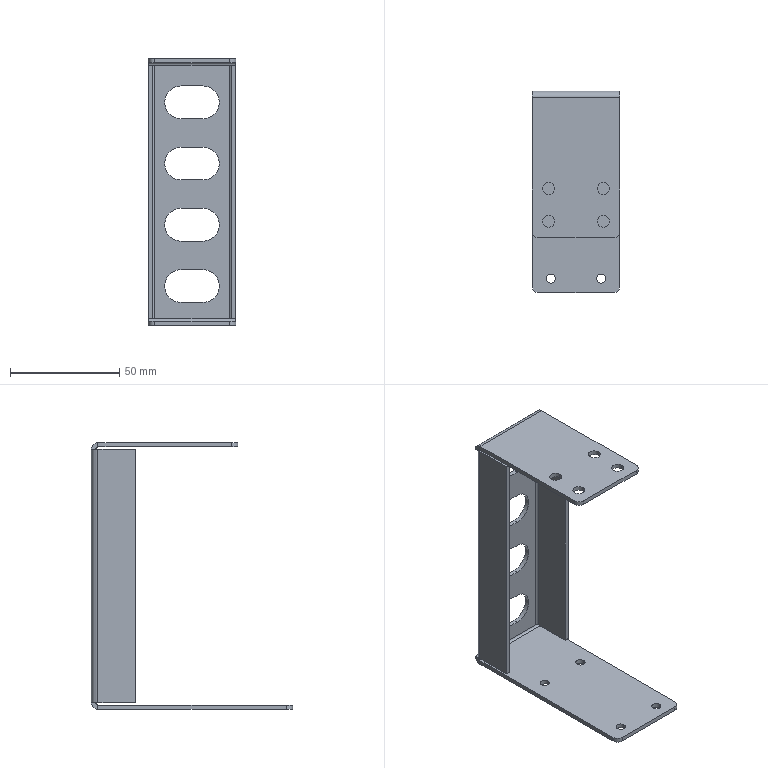Part | SolidWorks | features HoleWzd 2, EdgeFlange 1, Fillet 1, FlatPattern 1, ICE 1, LPattern 1, SMBaseFlange 1, SheetMetal 1 | 1 solid | 78 faces | box 40 x 92 x 122 mm | volume 27046 mm3 | plane 42 | cylinder 36 | commonest cylinder face diameters 4.2 x8 5.5 x8 6 x8 15 x8 2 x4